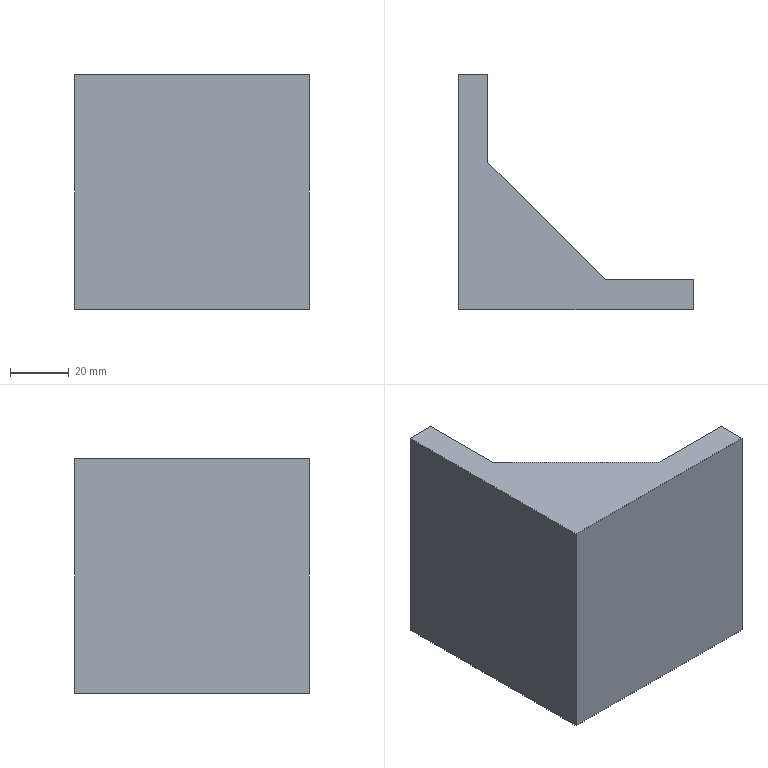Part | NX | features BREP 1 | 1 solid | 12 faces | box 80 x 80 x 80 mm | volume 136000 mm3 | plane 12
STEP:
#1=CARTESIAN_POINT('',(-80.,0.,80.));
#2=VERTEX_POINT('',#1);
#3=CARTESIAN_POINT('',(-80.,0.,0.));
#4=VERTEX_POINT('',#3);
#5=CARTESIAN_POINT('',(-80.,0.,80.));
#6=DIRECTION('',(0.,0.,-1.));
#7=VECTOR('',#6,1000.);
#8=LINE('',#5,#7);
#9=EDGE_CURVE('',#2,#4,#8,.T.);
#10=ORIENTED_EDGE('',*,*,#9,.F.);
#11=CARTESIAN_POINT('',(-80.,80.,80.));
#12=VERTEX_POINT('',#11);
#13=CARTESIAN_POINT('',(-80.,80.,80.));
#14=DIRECTION('',(0.,-1.,0.));
#15=VECTOR('',#14,1000.);
#16=LINE('',#13,#15);
#17=EDGE_CURVE('',#12,#2,#16,.T.);
#18=ORIENTED_EDGE('',*,*,#17,.F.);
#19=CARTESIAN_POINT('',(-80.,80.,0.));
#20=VERTEX_POINT('',#19);
#21=CARTESIAN_POINT('',(-80.,80.,80.));
#22=DIRECTION('',(0.,0.,1.));
#23=VECTOR('',#22,1000.);
#24=LINE('',#21,#23);
#25=EDGE_CURVE('',#20,#12,#24,.T.);
#26=ORIENTED_EDGE('',*,*,#25,.F.);
#27=CARTESIAN_POINT('',(-80.,80.,0.));
#28=DIRECTION('',(0.,1.,0.));
#29=VECTOR('',#28,1000.);
#30=LINE('',#27,#29);
#31=EDGE_CURVE('',#4,#20,#30,.T.);
#32=ORIENTED_EDGE('',*,*,#31,.F.);
#33=EDGE_LOOP('',(#10,#18,#26,#32));
#34=FACE_BOUND('',#33,.T.);
#35=CARTESIAN_POINT('',(-80.,80.,80.));
#36=DIRECTION('',(1.,0.,0.));
#37=DIRECTION('',(0.,1.,0.));
#38=AXIS2_PLACEMENT_3D('',#35,#36,#37);
#39=PLANE('',#38);
#40=ADVANCED_FACE('',(#34),#39,.F.);
#41=CARTESIAN_POINT('',(0.,10.,0.));
#42=VERTEX_POINT('',#41);
#43=CARTESIAN_POINT('',(-30.,10.,0.));
#44=VERTEX_POINT('',#43);
#45=CARTESIAN_POINT('',(-80.,10.,0.));
#46=DIRECTION('',(-1.,0.,0.));
#47=VECTOR('',#46,1000.);
#48=LINE('',#45,#47);
#49=EDGE_CURVE('',#42,#44,#48,.T.);
#50=ORIENTED_EDGE('',*,*,#49,.F.);
#51=CARTESIAN_POINT('',(0.,0.,0.));
#52=VERTEX_POINT('',#51);
#53=CARTESIAN_POINT('',(0.,0.,0.));
#54=DIRECTION('',(0.,1.,0.));
#55=VECTOR('',#54,1000.);
#56=LINE('',#53,#55);
#57=EDGE_CURVE('',#52,#42,#56,.T.);
#58=ORIENTED_EDGE('',*,*,#57,.F.);
#59=CARTESIAN_POINT('',(-80.,0.,0.));
#60=DIRECTION('',(1.,0.,0.));
#61=VECTOR('',#60,1000.);
#62=LINE('',#59,#61);
#63=EDGE_CURVE('',#4,#52,#62,.T.);
#64=ORIENTED_EDGE('',*,*,#63,.F.);
#65=ORIENTED_EDGE('',*,*,#31,.T.);
#66=CARTESIAN_POINT('',(-70.,80.,0.));
#67=VERTEX_POINT('',#66);
#68=CARTESIAN_POINT('',(-80.,80.,0.));
#69=DIRECTION('',(-1.,0.,0.));
#70=VECTOR('',#69,1000.);
#71=LINE('',#68,#70);
#72=EDGE_CURVE('',#67,#20,#71,.T.);
#73=ORIENTED_EDGE('',*,*,#72,.F.);
#74=CARTESIAN_POINT('',(-70.,50.,0.));
#75=VERTEX_POINT('',#74);
#76=CARTESIAN_POINT('',(-70.,0.,0.));
#77=DIRECTION('',(0.,1.,0.));
#78=VECTOR('',#77,1000.);
#79=LINE('',#76,#78);
#80=EDGE_CURVE('',#75,#67,#79,.T.);
#81=ORIENTED_EDGE('',*,*,#80,.F.);
#82=CARTESIAN_POINT('',(-30.,10.,0.));
#83=DIRECTION('',(-0.7071,0.7071,0.));
#84=VECTOR('',#83,1000.);
#85=LINE('',#82,#84);
#86=EDGE_CURVE('',#44,#75,#85,.T.);
#87=ORIENTED_EDGE('',*,*,#86,.F.);
#88=EDGE_LOOP('',(#50,#58,#64,#65,#73,#81,#87));
#89=FACE_BOUND('',#88,.T.);
#90=CARTESIAN_POINT('',(-80.,0.,0.));
#91=DIRECTION('',(0.,0.,1.));
#92=DIRECTION('',(1.,0.,0.));
#93=AXIS2_PLACEMENT_3D('',#90,#91,#92);
#94=PLANE('',#93);
#95=ADVANCED_FACE('',(#89),#94,.F.);
#96=CARTESIAN_POINT('',(0.,0.,80.));
#97=VERTEX_POINT('',#96);
#98=CARTESIAN_POINT('',(0.,0.,80.));
#99=DIRECTION('',(0.,0.,-1.));
#100=VECTOR('',#99,1000.);
#101=LINE('',#98,#100);
#102=EDGE_CURVE('',#97,#52,#101,.T.);
#103=ORIENTED_EDGE('',*,*,#102,.F.);
#104=CARTESIAN_POINT('',(-80.,0.,80.));
#105=DIRECTION('',(1.,0.,0.));
#106=VECTOR('',#105,1000.);
#107=LINE('',#104,#106);
#108=EDGE_CURVE('',#2,#97,#107,.T.);
#109=ORIENTED_EDGE('',*,*,#108,.F.);
#110=ORIENTED_EDGE('',*,*,#9,.T.);
#111=ORIENTED_EDGE('',*,*,#63,.T.);
#112=EDGE_LOOP('',(#103,#109,#110,#111));
#113=FACE_BOUND('',#112,.T.);
#114=CARTESIAN_POINT('',(-80.,0.,80.));
#115=DIRECTION('',(0.,1.,0.));
#116=DIRECTION('',(1.,0.,0.));
#117=AXIS2_PLACEMENT_3D('',#114,#115,#116);
#118=PLANE('',#117);
#119=ADVANCED_FACE('',(#113),#118,.F.);
#120=ORIENTED_EDGE('',*,*,#108,.T.);
#121=CARTESIAN_POINT('',(0.,10.,80.));
#122=VERTEX_POINT('',#121);
#123=CARTESIAN_POINT('',(0.,0.,80.));
#124=DIRECTION('',(0.,1.,0.));
#125=VECTOR('',#124,1000.);
#126=LINE('',#123,#125);
#127=EDGE_CURVE('',#97,#122,#126,.T.);
#128=ORIENTED_EDGE('',*,*,#127,.T.);
#129=CARTESIAN_POINT('',(-30.,10.,80.));
#130=VERTEX_POINT('',#129);
#131=CARTESIAN_POINT('',(-80.,10.,80.));
#132=DIRECTION('',(-1.,0.,0.));
#133=VECTOR('',#132,1000.);
#134=LINE('',#131,#133);
#135=EDGE_CURVE('',#122,#130,#134,.T.);
#136=ORIENTED_EDGE('',*,*,#135,.T.);
#137=CARTESIAN_POINT('',(-70.,50.,80.));
#138=VERTEX_POINT('',#137);
#139=CARTESIAN_POINT('',(-30.,10.,80.));
#140=DIRECTION('',(-0.7071,0.7071,0.));
#141=VECTOR('',#140,1000.);
#142=LINE('',#139,#141);
#143=EDGE_CURVE('',#130,#138,#142,.T.);
#144=ORIENTED_EDGE('',*,*,#143,.T.);
#145=CARTESIAN_POINT('',(-70.,80.,80.));
#146=VERTEX_POINT('',#145);
#147=CARTESIAN_POINT('',(-70.,0.,80.));
#148=DIRECTION('',(0.,1.,0.));
#149=VECTOR('',#148,1000.);
#150=LINE('',#147,#149);
#151=EDGE_CURVE('',#138,#146,#150,.T.);
#152=ORIENTED_EDGE('',*,*,#151,.T.);
#153=CARTESIAN_POINT('',(-80.,80.,80.));
#154=DIRECTION('',(-1.,0.,0.));
#155=VECTOR('',#154,1000.);
#156=LINE('',#153,#155);
#157=EDGE_CURVE('',#146,#12,#156,.T.);
#158=ORIENTED_EDGE('',*,*,#157,.T.);
#159=ORIENTED_EDGE('',*,*,#17,.T.);
#160=EDGE_LOOP('',(#120,#128,#136,#144,#152,#158,#159));
#161=FACE_BOUND('',#160,.T.);
#162=CARTESIAN_POINT('',(-80.,0.,80.));
#163=DIRECTION('',(0.,0.,1.));
#164=DIRECTION('',(1.,0.,0.));
#165=AXIS2_PLACEMENT_3D('',#162,#163,#164);
#166=PLANE('',#165);
#167=ADVANCED_FACE('',(#161),#166,.T.);
#168=CARTESIAN_POINT('',(-70.,80.,80.));
#169=DIRECTION('',(0.,0.,1.));
#170=VECTOR('',#169,1000.);
#171=LINE('',#168,#170);
#172=EDGE_CURVE('',#67,#146,#171,.T.);
#173=ORIENTED_EDGE('',*,*,#172,.F.);
#174=ORIENTED_EDGE('',*,*,#72,.T.);
#175=ORIENTED_EDGE('',*,*,#25,.T.);
#176=ORIENTED_EDGE('',*,*,#157,.F.);
#177=EDGE_LOOP('',(#173,#174,#175,#176));
#178=FACE_BOUND('',#177,.T.);
#179=CARTESIAN_POINT('',(-80.,80.,80.));
#180=DIRECTION('',(0.,-1.,0.));
#181=DIRECTION('',(0.,0.,-1.));
#182=AXIS2_PLACEMENT_3D('',#179,#180,#181);
#183=PLANE('',#182);
#184=ADVANCED_FACE('',(#178),#183,.F.);
#185=CARTESIAN_POINT('',(-30.,10.,10.));
#186=VERTEX_POINT('',#185);
#187=CARTESIAN_POINT('',(-30.,10.,0.));
#188=DIRECTION('',(0.,0.,1.));
#189=VECTOR('',#188,1000.);
#190=LINE('',#187,#189);
#191=EDGE_CURVE('',#44,#186,#190,.T.);
#192=ORIENTED_EDGE('',*,*,#191,.F.);
#193=ORIENTED_EDGE('',*,*,#86,.T.);
#194=CARTESIAN_POINT('',(-70.,50.,10.));
#195=VERTEX_POINT('',#194);
#196=CARTESIAN_POINT('',(-70.,50.,0.));
#197=DIRECTION('',(0.,0.,-1.));
#198=VECTOR('',#197,1000.);
#199=LINE('',#196,#198);
#200=EDGE_CURVE('',#195,#75,#199,.T.);
#201=ORIENTED_EDGE('',*,*,#200,.F.);
#202=CARTESIAN_POINT('',(-70.,50.,10.));
#203=DIRECTION('',(-0.7071,0.7071,0.));
#204=VECTOR('',#203,1000.);
#205=LINE('',#202,#204);
#206=EDGE_CURVE('',#186,#195,#205,.T.);
#207=ORIENTED_EDGE('',*,*,#206,.F.);
#208=EDGE_LOOP('',(#192,#193,#201,#207));
#209=FACE_BOUND('',#208,.T.);
#210=CARTESIAN_POINT('',(-70.,50.,0.));
#211=DIRECTION('',(-0.7071,-0.7071,0.));
#212=DIRECTION('',(-0.7071,0.7071,0.));
#213=AXIS2_PLACEMENT_3D('',#210,#211,#212);
#214=PLANE('',#213);
#215=ADVANCED_FACE('',(#209),#214,.F.);
#216=CARTESIAN_POINT('',(-70.,10.,10.));
#217=VERTEX_POINT('',#216);
#218=CARTESIAN_POINT('',(-80.,10.,10.));
#219=DIRECTION('',(-1.,0.,0.));
#220=VECTOR('',#219,1000.);
#221=LINE('',#218,#220);
#222=EDGE_CURVE('',#186,#217,#221,.T.);
#223=ORIENTED_EDGE('',*,*,#222,.T.);
#224=CARTESIAN_POINT('',(-70.,10.,70.));
#225=VERTEX_POINT('',#224);
#226=CARTESIAN_POINT('',(-70.,10.,80.));
#227=DIRECTION('',(0.,0.,1.));
#228=VECTOR('',#227,1000.);
#229=LINE('',#226,#228);
#230=EDGE_CURVE('',#217,#225,#229,.T.);
#231=ORIENTED_EDGE('',*,*,#230,.T.);
#232=CARTESIAN_POINT('',(-30.,10.,70.));
#233=VERTEX_POINT('',#232);
#234=CARTESIAN_POINT('',(-80.,10.,70.));
#235=DIRECTION('',(1.,0.,0.));
#236=VECTOR('',#235,1000.);
#237=LINE('',#234,#236);
#238=EDGE_CURVE('',#225,#233,#237,.T.);
#239=ORIENTED_EDGE('',*,*,#238,.T.);
#240=CARTESIAN_POINT('',(-30.,10.,80.));
#241=DIRECTION('',(0.,0.,1.));
#242=VECTOR('',#241,1000.);
#243=LINE('',#240,#242);
#244=EDGE_CURVE('',#233,#130,#243,.T.);
#245=ORIENTED_EDGE('',*,*,#244,.T.);
#246=ORIENTED_EDGE('',*,*,#135,.F.);
#247=CARTESIAN_POINT('',(0.,10.,80.));
#248=DIRECTION('',(0.,0.,-1.));
#249=VECTOR('',#248,1000.);
#250=LINE('',#247,#249);
#251=EDGE_CURVE('',#122,#42,#250,.T.);
#252=ORIENTED_EDGE('',*,*,#251,.T.);
#253=ORIENTED_EDGE('',*,*,#49,.T.);
#254=ORIENTED_EDGE('',*,*,#191,.T.);
#255=EDGE_LOOP('',(#223,#231,#239,#245,#246,#252,#253,#254));
#256=FACE_BOUND('',#255,.T.);
#257=CARTESIAN_POINT('',(-80.,10.,80.));
#258=DIRECTION('',(0.,1.,0.));
#259=DIRECTION('',(1.,0.,0.));
#260=AXIS2_PLACEMENT_3D('',#257,#258,#259);
#261=PLANE('',#260);
#262=ADVANCED_FACE('',(#256),#261,.T.);
#263=ORIENTED_EDGE('',*,*,#251,.F.);
#264=ORIENTED_EDGE('',*,*,#127,.F.);
#265=ORIENTED_EDGE('',*,*,#102,.T.);
#266=ORIENTED_EDGE('',*,*,#57,.T.);
#267=EDGE_LOOP('',(#263,#264,#265,#266));
#268=FACE_BOUND('',#267,.T.);
#269=CARTESIAN_POINT('',(0.,80.,80.));
#270=DIRECTION('',(-1.,0.,0.));
#271=DIRECTION('',(0.,1.,0.));
#272=AXIS2_PLACEMENT_3D('',#269,#270,#271);
#273=PLANE('',#272);
#274=ADVANCED_FACE('',(#268),#273,.F.);
#275=CARTESIAN_POINT('',(-70.,50.,70.));
#276=VERTEX_POINT('',#275);
#277=CARTESIAN_POINT('',(-70.,80.,70.));
#278=DIRECTION('',(0.,-1.,0.));
#279=VECTOR('',#278,1000.);
#280=LINE('',#277,#279);
#281=EDGE_CURVE('',#276,#225,#280,.T.);
#282=ORIENTED_EDGE('',*,*,#281,.T.);
#283=ORIENTED_EDGE('',*,*,#230,.F.);
#284=CARTESIAN_POINT('',(-70.,80.,10.));
#285=DIRECTION('',(0.,1.,0.));
#286=VECTOR('',#285,1000.);
#287=LINE('',#284,#286);
#288=EDGE_CURVE('',#217,#195,#287,.T.);
#289=ORIENTED_EDGE('',*,*,#288,.T.);
#290=ORIENTED_EDGE('',*,*,#200,.T.);
#291=ORIENTED_EDGE('',*,*,#80,.T.);
#292=ORIENTED_EDGE('',*,*,#172,.T.);
#293=ORIENTED_EDGE('',*,*,#151,.F.);
#294=CARTESIAN_POINT('',(-70.,50.,80.));
#295=DIRECTION('',(0.,0.,-1.));
#296=VECTOR('',#295,1000.);
#297=LINE('',#294,#296);
#298=EDGE_CURVE('',#138,#276,#297,.T.);
#299=ORIENTED_EDGE('',*,*,#298,.T.);
#300=EDGE_LOOP('',(#282,#283,#289,#290,#291,#292,#293,#299));
#301=FACE_BOUND('',#300,.T.);
#302=CARTESIAN_POINT('',(-70.,80.,80.));
#303=DIRECTION('',(1.,0.,0.));
#304=DIRECTION('',(0.,1.,0.));
#305=AXIS2_PLACEMENT_3D('',#302,#303,#304);
#306=PLANE('',#305);
#307=ADVANCED_FACE('',(#301),#306,.T.);
#308=ORIENTED_EDGE('',*,*,#143,.F.);
#309=ORIENTED_EDGE('',*,*,#244,.F.);
#310=CARTESIAN_POINT('',(-70.,50.,70.));
#311=DIRECTION('',(0.7071,-0.7071,0.));
#312=VECTOR('',#311,1000.);
#313=LINE('',#310,#312);
#314=EDGE_CURVE('',#276,#233,#313,.T.);
#315=ORIENTED_EDGE('',*,*,#314,.F.);
#316=ORIENTED_EDGE('',*,*,#298,.F.);
#317=EDGE_LOOP('',(#308,#309,#315,#316));
#318=FACE_BOUND('',#317,.T.);
#319=CARTESIAN_POINT('',(-70.,50.,0.));
#320=DIRECTION('',(-0.7071,-0.7071,0.));
#321=DIRECTION('',(-0.7071,0.7071,0.));
#322=AXIS2_PLACEMENT_3D('',#319,#320,#321);
#323=PLANE('',#322);
#324=ADVANCED_FACE('',(#318),#323,.F.);
#325=ORIENTED_EDGE('',*,*,#288,.F.);
#326=ORIENTED_EDGE('',*,*,#222,.F.);
#327=ORIENTED_EDGE('',*,*,#206,.T.);
#328=EDGE_LOOP('',(#325,#326,#327));
#329=FACE_BOUND('',#328,.T.);
#330=CARTESIAN_POINT('',(-80.,0.,10.));
#331=DIRECTION('',(0.,0.,1.));
#332=DIRECTION('',(1.,0.,0.));
#333=AXIS2_PLACEMENT_3D('',#330,#331,#332);
#334=PLANE('',#333);
#335=ADVANCED_FACE('',(#329),#334,.T.);
#336=ORIENTED_EDGE('',*,*,#314,.T.);
#337=ORIENTED_EDGE('',*,*,#238,.F.);
#338=ORIENTED_EDGE('',*,*,#281,.F.);
#339=EDGE_LOOP('',(#336,#337,#338));
#340=FACE_BOUND('',#339,.T.);
#341=CARTESIAN_POINT('',(-80.,0.,70.));
#342=DIRECTION('',(0.,0.,1.));
#343=DIRECTION('',(1.,0.,0.));
#344=AXIS2_PLACEMENT_3D('',#341,#342,#343);
#345=PLANE('',#344);
#346=ADVANCED_FACE('',(#340),#345,.F.);
#347=CLOSED_SHELL('',(#40,#95,#119,#167,#184,#215,#262,#274,#307,#324,#335,#346));
#348=MANIFOLD_SOLID_BREP('',#347);
#349=(LENGTH_UNIT()NAMED_UNIT(*)SI_UNIT(.MILLI.,.METRE.));
#350=UNCERTAINTY_MEASURE_WITH_UNIT(LENGTH_MEASURE(0.00001),#349,'','');
#351=(NAMED_UNIT(*)PLANE_ANGLE_UNIT()SI_UNIT($,.RADIAN.));
#352=(NAMED_UNIT(*)SI_UNIT($,.STERADIAN.)SOLID_ANGLE_UNIT());
#353=(GEOMETRIC_REPRESENTATION_CONTEXT(3)GLOBAL_UNCERTAINTY_ASSIGNED_CONTEXT((#350))GLOBAL_UNIT_ASSIGNED_CONTEXT((#349,#351,#352))REPRESENTATION_CONTEXT('',''));
#354=ADVANCED_BREP_SHAPE_REPRESENTATION('',(#348),#353);